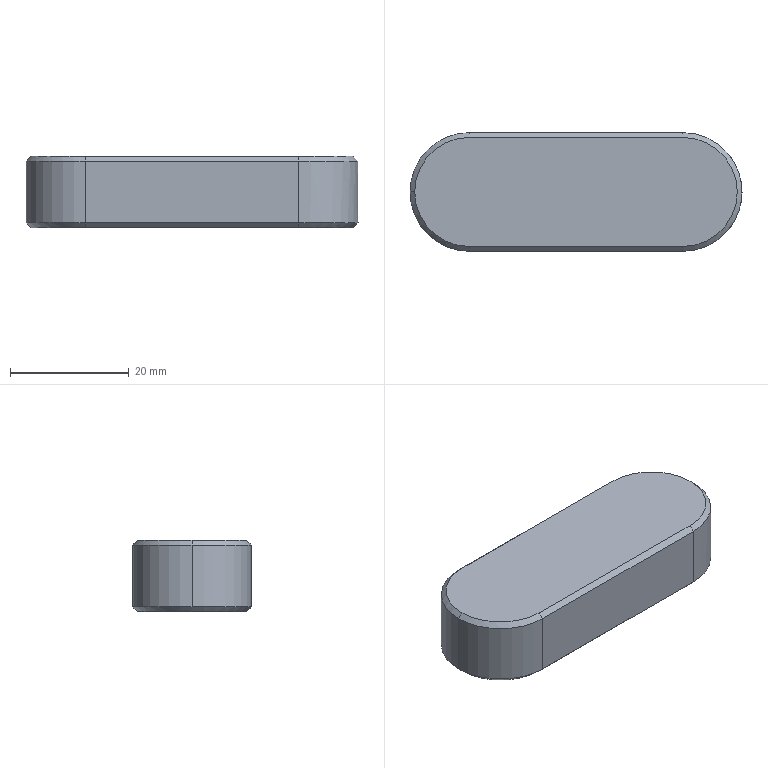Part | SolidWorks | features Boss 2, Chamfer 1, Extrusion 1 | 1 solid | 17 faces | box 56 x 20 x 12 mm | volume 12325 mm3 | plane 8 | cone 6 | cylinder 3 | commonest cylinder face diameters 20 x3
STEP:
#1=CARTESIAN_POINT('',(-45.2,0.,6.));
#2=VERTEX_POINT('',#1);
#3=CARTESIAN_POINT('',(-36.,-9.2,6.));
#4=VERTEX_POINT('',#3);
#5=CARTESIAN_POINT('',(-36.,0.,6.));
#6=DIRECTION('',(0.,0.,1.));
#7=DIRECTION('',(-1.,0.,0.));
#8=AXIS2_PLACEMENT_3D('',#5,#6,#7);
#9=CIRCLE('',#8,9.2);
#10=EDGE_CURVE('',#2,#4,#9,.T.);
#11=ORIENTED_EDGE('',*,*,#10,.F.);
#12=CARTESIAN_POINT('',(-46.,0.,5.2));
#13=VERTEX_POINT('',#12);
#14=CARTESIAN_POINT('',(-45.2,0.,6.));
#15=DIRECTION('',(-0.7071,0.,-0.7071));
#16=VECTOR('',#15,1000.);
#17=LINE('',#14,#16);
#18=EDGE_CURVE('',#2,#13,#17,.T.);
#19=ORIENTED_EDGE('',*,*,#18,.T.);
#20=CARTESIAN_POINT('',(-36.,-10.,5.2));
#21=VERTEX_POINT('',#20);
#22=CARTESIAN_POINT('',(-36.,0.,5.2));
#23=DIRECTION('',(0.,0.,-1.));
#24=DIRECTION('',(-1.,0.,0.));
#25=AXIS2_PLACEMENT_3D('',#22,#23,#24);
#26=CIRCLE('',#25,10.);
#27=EDGE_CURVE('',#21,#13,#26,.T.);
#28=ORIENTED_EDGE('',*,*,#27,.F.);
#29=CARTESIAN_POINT('',(-36.,-9.2,6.));
#30=DIRECTION('',(0.,-0.7071,-0.7071));
#31=VECTOR('',#30,1000.);
#32=LINE('',#29,#31);
#33=EDGE_CURVE('',#4,#21,#32,.T.);
#34=ORIENTED_EDGE('',*,*,#33,.F.);
#35=EDGE_LOOP('',(#11,#19,#28,#34));
#36=FACE_OUTER_BOUND('',#35,.T.);
#37=CARTESIAN_POINT('',(-36.,0.,6.));
#38=DIRECTION('',(0.,0.,-1.));
#39=DIRECTION('',(-1.,0.,0.));
#40=AXIS2_PLACEMENT_3D('',#37,#38,#39);
#41=CONICAL_SURFACE('',#40,9.2,0.7854);
#42=ADVANCED_FACE('',(#36),#41,.T.);
#43=CARTESIAN_POINT('',(9.2,0.,-6.));
#44=VERTEX_POINT('',#43);
#45=CARTESIAN_POINT('',(0.,-9.2,-6.));
#46=VERTEX_POINT('',#45);
#47=CARTESIAN_POINT('',(0.,0.,-6.));
#48=DIRECTION('',(0.,0.,-1.));
#49=DIRECTION('',(-1.,0.,0.));
#50=AXIS2_PLACEMENT_3D('',#47,#48,#49);
#51=CIRCLE('',#50,9.2);
#52=EDGE_CURVE('',#44,#46,#51,.T.);
#53=ORIENTED_EDGE('',*,*,#52,.F.);
#54=CARTESIAN_POINT('',(10.,0.,-5.2));
#55=VERTEX_POINT('',#54);
#56=CARTESIAN_POINT('',(10.,0.,-5.2));
#57=DIRECTION('',(0.7071,0.,0.7071));
#58=VECTOR('',#57,1000.);
#59=LINE('',#56,#58);
#60=EDGE_CURVE('',#44,#55,#59,.T.);
#61=ORIENTED_EDGE('',*,*,#60,.T.);
#62=CARTESIAN_POINT('',(0.,-10.,-5.2));
#63=VERTEX_POINT('',#62);
#64=CARTESIAN_POINT('',(0.,0.,-5.2));
#65=DIRECTION('',(0.,0.,1.));
#66=DIRECTION('',(-1.,0.,0.));
#67=AXIS2_PLACEMENT_3D('',#64,#65,#66);
#68=CIRCLE('',#67,10.);
#69=EDGE_CURVE('',#63,#55,#68,.T.);
#70=ORIENTED_EDGE('',*,*,#69,.F.);
#71=CARTESIAN_POINT('',(0.,-9.2,-6.));
#72=DIRECTION('',(0.,-0.7071,0.7071));
#73=VECTOR('',#72,1000.);
#74=LINE('',#71,#73);
#75=EDGE_CURVE('',#46,#63,#74,.T.);
#76=ORIENTED_EDGE('',*,*,#75,.F.);
#77=EDGE_LOOP('',(#53,#61,#70,#76));
#78=FACE_OUTER_BOUND('',#77,.T.);
#79=CARTESIAN_POINT('',(0.,0.,-5.2));
#80=DIRECTION('',(0.,0.,1.));
#81=DIRECTION('',(1.,0.,0.));
#82=AXIS2_PLACEMENT_3D('',#79,#80,#81);
#83=CONICAL_SURFACE('',#82,10.,0.7854);
#84=ADVANCED_FACE('',(#78),#83,.T.);
#85=ORIENTED_EDGE('',*,*,#27,.T.);
#86=CARTESIAN_POINT('',(-46.,0.,-5.2));
#87=VERTEX_POINT('',#86);
#88=CARTESIAN_POINT('',(-46.,0.,6.));
#89=DIRECTION('',(0.,0.,-1.));
#90=VECTOR('',#89,1000.);
#91=LINE('',#88,#90);
#92=EDGE_CURVE('',#13,#87,#91,.T.);
#93=ORIENTED_EDGE('',*,*,#92,.T.);
#94=CARTESIAN_POINT('',(-36.,-10.,-5.2));
#95=VERTEX_POINT('',#94);
#96=CARTESIAN_POINT('',(-36.,0.,-5.2));
#97=DIRECTION('',(0.,0.,1.));
#98=DIRECTION('',(-1.,0.,0.));
#99=AXIS2_PLACEMENT_3D('',#96,#97,#98);
#100=CIRCLE('',#99,10.);
#101=EDGE_CURVE('',#87,#95,#100,.T.);
#102=ORIENTED_EDGE('',*,*,#101,.T.);
#103=CARTESIAN_POINT('',(-36.,-10.,6.));
#104=DIRECTION('',(0.,0.,-1.));
#105=VECTOR('',#104,1000.);
#106=LINE('',#103,#105);
#107=EDGE_CURVE('',#21,#95,#106,.T.);
#108=ORIENTED_EDGE('',*,*,#107,.F.);
#109=EDGE_LOOP('',(#85,#93,#102,#108));
#110=FACE_OUTER_BOUND('',#109,.T.);
#111=CARTESIAN_POINT('',(-36.,0.,6.));
#112=DIRECTION('',(0.,0.,-1.));
#113=DIRECTION('',(-1.,0.,0.));
#114=AXIS2_PLACEMENT_3D('',#111,#112,#113);
#115=CYLINDRICAL_SURFACE('',#114,10.);
#116=ADVANCED_FACE('',(#110),#115,.T.);
#117=ORIENTED_EDGE('',*,*,#92,.F.);
#118=CARTESIAN_POINT('',(-36.,10.,5.2));
#119=VERTEX_POINT('',#118);
#120=CARTESIAN_POINT('',(-36.,0.,5.2));
#121=DIRECTION('',(0.,0.,-1.));
#122=DIRECTION('',(-1.,0.,0.));
#123=AXIS2_PLACEMENT_3D('',#120,#121,#122);
#124=CIRCLE('',#123,10.);
#125=EDGE_CURVE('',#13,#119,#124,.T.);
#126=ORIENTED_EDGE('',*,*,#125,.T.);
#127=CARTESIAN_POINT('',(-36.,10.,-5.2));
#128=VERTEX_POINT('',#127);
#129=CARTESIAN_POINT('',(-36.,10.,6.));
#130=DIRECTION('',(0.,0.,-1.));
#131=VECTOR('',#130,1000.);
#132=LINE('',#129,#131);
#133=EDGE_CURVE('',#119,#128,#132,.T.);
#134=ORIENTED_EDGE('',*,*,#133,.T.);
#135=CARTESIAN_POINT('',(-36.,0.,-5.2));
#136=DIRECTION('',(0.,0.,1.));
#137=DIRECTION('',(-1.,0.,0.));
#138=AXIS2_PLACEMENT_3D('',#135,#136,#137);
#139=CIRCLE('',#138,10.);
#140=EDGE_CURVE('',#128,#87,#139,.T.);
#141=ORIENTED_EDGE('',*,*,#140,.T.);
#142=EDGE_LOOP('',(#117,#126,#134,#141));
#143=FACE_OUTER_BOUND('',#142,.T.);
#144=CARTESIAN_POINT('',(-36.,0.,6.));
#145=DIRECTION('',(0.,0.,-1.));
#146=DIRECTION('',(-1.,0.,0.));
#147=AXIS2_PLACEMENT_3D('',#144,#145,#146);
#148=CYLINDRICAL_SURFACE('',#147,10.);
#149=ADVANCED_FACE('',(#143),#148,.T.);
#150=ORIENTED_EDGE('',*,*,#107,.T.);
#151=CARTESIAN_POINT('',(0.,-10.,-5.2));
#152=DIRECTION('',(1.,0.,0.));
#153=VECTOR('',#152,1000.);
#154=LINE('',#151,#153);
#155=EDGE_CURVE('',#95,#63,#154,.T.);
#156=ORIENTED_EDGE('',*,*,#155,.T.);
#157=CARTESIAN_POINT('',(0.,-10.,5.2));
#158=VERTEX_POINT('',#157);
#159=CARTESIAN_POINT('',(0.,-10.,6.));
#160=DIRECTION('',(0.,0.,-1.));
#161=VECTOR('',#160,1000.);
#162=LINE('',#159,#161);
#163=EDGE_CURVE('',#158,#63,#162,.T.);
#164=ORIENTED_EDGE('',*,*,#163,.F.);
#165=CARTESIAN_POINT('',(0.,-10.,5.2));
#166=DIRECTION('',(-1.,0.,0.));
#167=VECTOR('',#166,1000.);
#168=LINE('',#165,#167);
#169=EDGE_CURVE('',#158,#21,#168,.T.);
#170=ORIENTED_EDGE('',*,*,#169,.T.);
#171=EDGE_LOOP('',(#150,#156,#164,#170));
#172=FACE_OUTER_BOUND('',#171,.T.);
#173=CARTESIAN_POINT('',(0.,-10.,6.));
#174=DIRECTION('',(0.,1.,0.));
#175=DIRECTION('',(-1.,0.,0.));
#176=AXIS2_PLACEMENT_3D('',#173,#174,#175);
#177=PLANE('',#176);
#178=ADVANCED_FACE('',(#172),#177,.F.);
#179=CARTESIAN_POINT('',(0.,10.,5.2));
#180=VERTEX_POINT('',#179);
#181=CARTESIAN_POINT('',(0.,10.,-5.2));
#182=VERTEX_POINT('',#181);
#183=CARTESIAN_POINT('',(0.,10.,6.));
#184=DIRECTION('',(0.,0.,-1.));
#185=VECTOR('',#184,1000.);
#186=LINE('',#183,#185);
#187=EDGE_CURVE('',#180,#182,#186,.T.);
#188=ORIENTED_EDGE('',*,*,#187,.F.);
#189=CARTESIAN_POINT('',(0.,0.,5.2));
#190=DIRECTION('',(0.,0.,-1.));
#191=DIRECTION('',(-1.,0.,0.));
#192=AXIS2_PLACEMENT_3D('',#189,#190,#191);
#193=CIRCLE('',#192,10.);
#194=EDGE_CURVE('',#180,#158,#193,.T.);
#195=ORIENTED_EDGE('',*,*,#194,.T.);
#196=ORIENTED_EDGE('',*,*,#163,.T.);
#197=ORIENTED_EDGE('',*,*,#69,.T.);
#198=CARTESIAN_POINT('',(0.,0.,-5.2));
#199=DIRECTION('',(0.,0.,1.));
#200=DIRECTION('',(-1.,0.,0.));
#201=AXIS2_PLACEMENT_3D('',#198,#199,#200);
#202=CIRCLE('',#201,10.);
#203=EDGE_CURVE('',#55,#182,#202,.T.);
#204=ORIENTED_EDGE('',*,*,#203,.T.);
#205=EDGE_LOOP('',(#188,#195,#196,#197,#204));
#206=FACE_OUTER_BOUND('',#205,.T.);
#207=CARTESIAN_POINT('',(0.,0.,6.));
#208=DIRECTION('',(0.,0.,-1.));
#209=DIRECTION('',(-1.,0.,0.));
#210=AXIS2_PLACEMENT_3D('',#207,#208,#209);
#211=CYLINDRICAL_SURFACE('',#210,10.);
#212=ADVANCED_FACE('',(#206),#211,.T.);
#213=ORIENTED_EDGE('',*,*,#133,.F.);
#214=CARTESIAN_POINT('',(-36.,10.,5.2));
#215=DIRECTION('',(1.,0.,0.));
#216=VECTOR('',#215,1000.);
#217=LINE('',#214,#216);
#218=EDGE_CURVE('',#119,#180,#217,.T.);
#219=ORIENTED_EDGE('',*,*,#218,.T.);
#220=ORIENTED_EDGE('',*,*,#187,.T.);
#221=CARTESIAN_POINT('',(-36.,10.,-5.2));
#222=DIRECTION('',(-1.,0.,0.));
#223=VECTOR('',#222,1000.);
#224=LINE('',#221,#223);
#225=EDGE_CURVE('',#182,#128,#224,.T.);
#226=ORIENTED_EDGE('',*,*,#225,.T.);
#227=EDGE_LOOP('',(#213,#219,#220,#226));
#228=FACE_OUTER_BOUND('',#227,.T.);
#229=CARTESIAN_POINT('',(-36.,10.,6.));
#230=DIRECTION('',(0.,-1.,0.));
#231=DIRECTION('',(0.,0.,-1.));
#232=AXIS2_PLACEMENT_3D('',#229,#230,#231);
#233=PLANE('',#232);
#234=ADVANCED_FACE('',(#228),#233,.F.);
#235=CARTESIAN_POINT('',(-36.,9.2,6.));
#236=VERTEX_POINT('',#235);
#237=CARTESIAN_POINT('',(-36.,0.,6.));
#238=DIRECTION('',(0.,0.,1.));
#239=DIRECTION('',(-1.,0.,0.));
#240=AXIS2_PLACEMENT_3D('',#237,#238,#239);
#241=CIRCLE('',#240,9.2);
#242=EDGE_CURVE('',#236,#2,#241,.T.);
#243=ORIENTED_EDGE('',*,*,#242,.T.);
#244=ORIENTED_EDGE('',*,*,#10,.T.);
#245=CARTESIAN_POINT('',(0.,-9.2,6.));
#246=VERTEX_POINT('',#245);
#247=CARTESIAN_POINT('',(-36.,-9.2,6.));
#248=DIRECTION('',(1.,0.,0.));
#249=VECTOR('',#248,1000.);
#250=LINE('',#247,#249);
#251=EDGE_CURVE('',#4,#246,#250,.T.);
#252=ORIENTED_EDGE('',*,*,#251,.T.);
#253=CARTESIAN_POINT('',(0.,9.2,6.));
#254=VERTEX_POINT('',#253);
#255=CARTESIAN_POINT('',(0.,0.,6.));
#256=DIRECTION('',(0.,0.,1.));
#257=DIRECTION('',(-1.,0.,0.));
#258=AXIS2_PLACEMENT_3D('',#255,#256,#257);
#259=CIRCLE('',#258,9.2);
#260=EDGE_CURVE('',#246,#254,#259,.T.);
#261=ORIENTED_EDGE('',*,*,#260,.T.);
#262=CARTESIAN_POINT('',(-36.,9.2,6.));
#263=DIRECTION('',(-1.,0.,0.));
#264=VECTOR('',#263,1000.);
#265=LINE('',#262,#264);
#266=EDGE_CURVE('',#254,#236,#265,.T.);
#267=ORIENTED_EDGE('',*,*,#266,.T.);
#268=EDGE_LOOP('',(#243,#244,#252,#261,#267));
#269=FACE_OUTER_BOUND('',#268,.T.);
#270=CARTESIAN_POINT('',(-36.,0.,6.));
#271=DIRECTION('',(0.,0.,-1.));
#272=DIRECTION('',(-1.,0.,0.));
#273=AXIS2_PLACEMENT_3D('',#270,#271,#272);
#274=PLANE('',#273);
#275=ADVANCED_FACE('',(#269),#274,.F.);
#276=CARTESIAN_POINT('',(0.,9.2,-6.));
#277=VERTEX_POINT('',#276);
#278=CARTESIAN_POINT('',(0.,0.,-6.));
#279=DIRECTION('',(0.,0.,-1.));
#280=DIRECTION('',(-1.,0.,0.));
#281=AXIS2_PLACEMENT_3D('',#278,#279,#280);
#282=CIRCLE('',#281,9.2);
#283=EDGE_CURVE('',#277,#44,#282,.T.);
#284=ORIENTED_EDGE('',*,*,#283,.T.);
#285=ORIENTED_EDGE('',*,*,#52,.T.);
#286=CARTESIAN_POINT('',(-36.,-9.2,-6.));
#287=VERTEX_POINT('',#286);
#288=CARTESIAN_POINT('',(-36.,-9.2,-6.));
#289=DIRECTION('',(-1.,0.,0.));
#290=VECTOR('',#289,1000.);
#291=LINE('',#288,#290);
#292=EDGE_CURVE('',#46,#287,#291,.T.);
#293=ORIENTED_EDGE('',*,*,#292,.T.);
#294=CARTESIAN_POINT('',(-36.,9.2,-6.));
#295=VERTEX_POINT('',#294);
#296=CARTESIAN_POINT('',(-36.,0.,-6.));
#297=DIRECTION('',(0.,0.,-1.));
#298=DIRECTION('',(-1.,0.,0.));
#299=AXIS2_PLACEMENT_3D('',#296,#297,#298);
#300=CIRCLE('',#299,9.2);
#301=EDGE_CURVE('',#287,#295,#300,.T.);
#302=ORIENTED_EDGE('',*,*,#301,.T.);
#303=CARTESIAN_POINT('',(0.,9.2,-6.));
#304=DIRECTION('',(1.,0.,0.));
#305=VECTOR('',#304,1000.);
#306=LINE('',#303,#305);
#307=EDGE_CURVE('',#295,#277,#306,.T.);
#308=ORIENTED_EDGE('',*,*,#307,.T.);
#309=EDGE_LOOP('',(#284,#285,#293,#302,#308));
#310=FACE_OUTER_BOUND('',#309,.T.);
#311=CARTESIAN_POINT('',(-36.,0.,-6.));
#312=DIRECTION('',(0.,0.,-1.));
#313=DIRECTION('',(-1.,0.,0.));
#314=AXIS2_PLACEMENT_3D('',#311,#312,#313);
#315=PLANE('',#314);
#316=ADVANCED_FACE('',(#310),#315,.T.);
#317=CARTESIAN_POINT('',(0.,9.2,-6.));
#318=DIRECTION('',(0.,0.7071,0.7071));
#319=VECTOR('',#318,1000.);
#320=LINE('',#317,#319);
#321=EDGE_CURVE('',#277,#182,#320,.T.);
#322=ORIENTED_EDGE('',*,*,#321,.F.);
#323=ORIENTED_EDGE('',*,*,#307,.F.);
#324=CARTESIAN_POINT('',(-36.,10.,-5.2));
#325=DIRECTION('',(0.,-0.7071,-0.7071));
#326=VECTOR('',#325,1000.);
#327=LINE('',#324,#326);
#328=EDGE_CURVE('',#128,#295,#327,.T.);
#329=ORIENTED_EDGE('',*,*,#328,.F.);
#330=ORIENTED_EDGE('',*,*,#225,.F.);
#331=EDGE_LOOP('',(#322,#323,#329,#330));
#332=FACE_OUTER_BOUND('',#331,.T.);
#333=CARTESIAN_POINT('',(-36.,10.,-5.2));
#334=DIRECTION('',(0.,0.7071,-0.7071));
#335=DIRECTION('',(0.,0.7071,0.7071));
#336=AXIS2_PLACEMENT_3D('',#333,#334,#335);
#337=PLANE('',#336);
#338=ADVANCED_FACE('',(#332),#337,.T.);
#339=ORIENTED_EDGE('',*,*,#328,.T.);
#340=ORIENTED_EDGE('',*,*,#301,.F.);
#341=CARTESIAN_POINT('',(-36.,-10.,-5.2));
#342=DIRECTION('',(0.,0.7071,-0.7071));
#343=VECTOR('',#342,1000.);
#344=LINE('',#341,#343);
#345=EDGE_CURVE('',#95,#287,#344,.T.);
#346=ORIENTED_EDGE('',*,*,#345,.F.);
#347=ORIENTED_EDGE('',*,*,#101,.F.);
#348=ORIENTED_EDGE('',*,*,#140,.F.);
#349=EDGE_LOOP('',(#339,#340,#346,#347,#348));
#350=FACE_OUTER_BOUND('',#349,.T.);
#351=CARTESIAN_POINT('',(-36.,0.,-5.2));
#352=DIRECTION('',(0.,0.,1.));
#353=DIRECTION('',(1.,0.,0.));
#354=AXIS2_PLACEMENT_3D('',#351,#352,#353);
#355=CONICAL_SURFACE('',#354,10.,0.7854);
#356=ADVANCED_FACE('',(#350),#355,.T.);
#357=ORIENTED_EDGE('',*,*,#60,.F.);
#358=ORIENTED_EDGE('',*,*,#283,.F.);
#359=ORIENTED_EDGE('',*,*,#321,.T.);
#360=ORIENTED_EDGE('',*,*,#203,.F.);
#361=EDGE_LOOP('',(#357,#358,#359,#360));
#362=FACE_OUTER_BOUND('',#361,.T.);
#363=CARTESIAN_POINT('',(0.,0.,-5.2));
#364=DIRECTION('',(0.,0.,1.));
#365=DIRECTION('',(1.,0.,0.));
#366=AXIS2_PLACEMENT_3D('',#363,#364,#365);
#367=CONICAL_SURFACE('',#366,10.,0.7854);
#368=ADVANCED_FACE('',(#362),#367,.T.);
#369=ORIENTED_EDGE('',*,*,#345,.T.);
#370=ORIENTED_EDGE('',*,*,#292,.F.);
#371=ORIENTED_EDGE('',*,*,#75,.T.);
#372=ORIENTED_EDGE('',*,*,#155,.F.);
#373=EDGE_LOOP('',(#369,#370,#371,#372));
#374=FACE_OUTER_BOUND('',#373,.T.);
#375=CARTESIAN_POINT('',(0.,-10.,-5.2));
#376=DIRECTION('',(0.,-0.7071,-0.7071));
#377=DIRECTION('',(0.,0.7071,-0.7071));
#378=AXIS2_PLACEMENT_3D('',#375,#376,#377);
#379=PLANE('',#378);
#380=ADVANCED_FACE('',(#374),#379,.T.);
#381=CARTESIAN_POINT('',(0.,10.,5.2));
#382=DIRECTION('',(0.,-0.7071,0.7071));
#383=VECTOR('',#382,1000.);
#384=LINE('',#381,#383);
#385=EDGE_CURVE('',#180,#254,#384,.T.);
#386=ORIENTED_EDGE('',*,*,#385,.F.);
#387=ORIENTED_EDGE('',*,*,#218,.F.);
#388=CARTESIAN_POINT('',(-36.,9.2,6.));
#389=DIRECTION('',(0.,0.7071,-0.7071));
#390=VECTOR('',#389,1000.);
#391=LINE('',#388,#390);
#392=EDGE_CURVE('',#236,#119,#391,.T.);
#393=ORIENTED_EDGE('',*,*,#392,.F.);
#394=ORIENTED_EDGE('',*,*,#266,.F.);
#395=EDGE_LOOP('',(#386,#387,#393,#394));
#396=FACE_OUTER_BOUND('',#395,.T.);
#397=CARTESIAN_POINT('',(-36.,9.2,6.));
#398=DIRECTION('',(0.,-0.7071,-0.7071));
#399=DIRECTION('',(0.,0.7071,-0.7071));
#400=AXIS2_PLACEMENT_3D('',#397,#398,#399);
#401=PLANE('',#400);
#402=ADVANCED_FACE('',(#396),#401,.F.);
#403=ORIENTED_EDGE('',*,*,#18,.F.);
#404=ORIENTED_EDGE('',*,*,#242,.F.);
#405=ORIENTED_EDGE('',*,*,#392,.T.);
#406=ORIENTED_EDGE('',*,*,#125,.F.);
#407=EDGE_LOOP('',(#403,#404,#405,#406));
#408=FACE_OUTER_BOUND('',#407,.T.);
#409=CARTESIAN_POINT('',(-36.,0.,6.));
#410=DIRECTION('',(0.,0.,-1.));
#411=DIRECTION('',(-1.,0.,0.));
#412=AXIS2_PLACEMENT_3D('',#409,#410,#411);
#413=CONICAL_SURFACE('',#412,9.2,0.7854);
#414=ADVANCED_FACE('',(#408),#413,.T.);
#415=ORIENTED_EDGE('',*,*,#385,.T.);
#416=ORIENTED_EDGE('',*,*,#260,.F.);
#417=CARTESIAN_POINT('',(0.,-10.,5.2));
#418=DIRECTION('',(0.,0.7071,0.7071));
#419=VECTOR('',#418,1000.);
#420=LINE('',#417,#419);
#421=EDGE_CURVE('',#158,#246,#420,.T.);
#422=ORIENTED_EDGE('',*,*,#421,.F.);
#423=ORIENTED_EDGE('',*,*,#194,.F.);
#424=EDGE_LOOP('',(#415,#416,#422,#423));
#425=FACE_OUTER_BOUND('',#424,.T.);
#426=CARTESIAN_POINT('',(0.,0.,6.));
#427=DIRECTION('',(0.,0.,-1.));
#428=DIRECTION('',(-1.,0.,0.));
#429=AXIS2_PLACEMENT_3D('',#426,#427,#428);
#430=CONICAL_SURFACE('',#429,9.2,0.7854);
#431=ADVANCED_FACE('',(#425),#430,.T.);
#432=ORIENTED_EDGE('',*,*,#33,.T.);
#433=ORIENTED_EDGE('',*,*,#169,.F.);
#434=ORIENTED_EDGE('',*,*,#421,.T.);
#435=ORIENTED_EDGE('',*,*,#251,.F.);
#436=EDGE_LOOP('',(#432,#433,#434,#435));
#437=FACE_OUTER_BOUND('',#436,.T.);
#438=CARTESIAN_POINT('',(-36.,-9.2,6.));
#439=DIRECTION('',(0.,0.7071,-0.7071));
#440=DIRECTION('',(0.,0.7071,0.7071));
#441=AXIS2_PLACEMENT_3D('',#438,#439,#440);
#442=PLANE('',#441);
#443=ADVANCED_FACE('',(#437),#442,.F.);
#444=CLOSED_SHELL('',(#42,#84,#116,#149,#178,#212,#234,#275,#316,#338,#356,#368,#380,#402,#414,#431,#443));
#445=MANIFOLD_SOLID_BREP('',#444);
#446=CARTESIAN_POINT('',(0.,0.,0.));
#447=DIRECTION('',(0.,0.,1.));
#448=DIRECTION('',(1.,0.,0.));
#449=AXIS2_PLACEMENT_3D('',#446,#447,#448);
#450=(LENGTH_UNIT()NAMED_UNIT(*)SI_UNIT(.MILLI.,.METRE.));
#451=UNCERTAINTY_MEASURE_WITH_UNIT(LENGTH_MEASURE(0.00001),#450,'','');
#452=(NAMED_UNIT(*)PLANE_ANGLE_UNIT()SI_UNIT($,.RADIAN.));
#453=(NAMED_UNIT(*)SI_UNIT($,.STERADIAN.)SOLID_ANGLE_UNIT());
#454=(GEOMETRIC_REPRESENTATION_CONTEXT(3)GLOBAL_UNCERTAINTY_ASSIGNED_CONTEXT((#451))GLOBAL_UNIT_ASSIGNED_CONTEXT((#450,#452,#453))REPRESENTATION_CONTEXT('',''));
#455=ADVANCED_BREP_SHAPE_REPRESENTATION('',(#445,#449),#454);